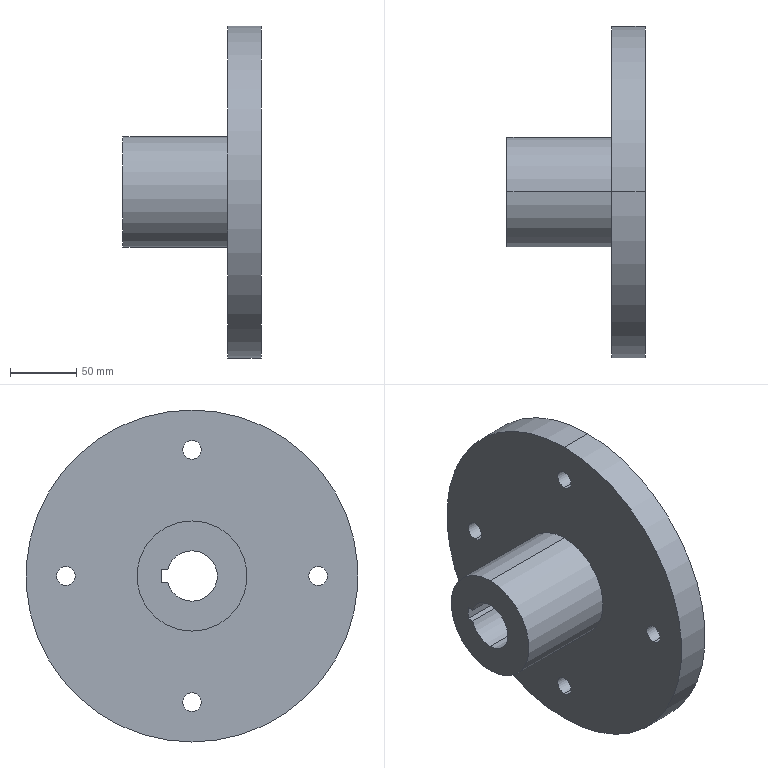Part | STEP file | Coupling 2 | 1 solid | 27 faces | box 104 x 250 x 250 mm | volume 1439037 mm3 | cylinder 19 | plane 8 | commonest cylinder face diameters 14 x8 83 x4 38 x3 96 x2 250 x2